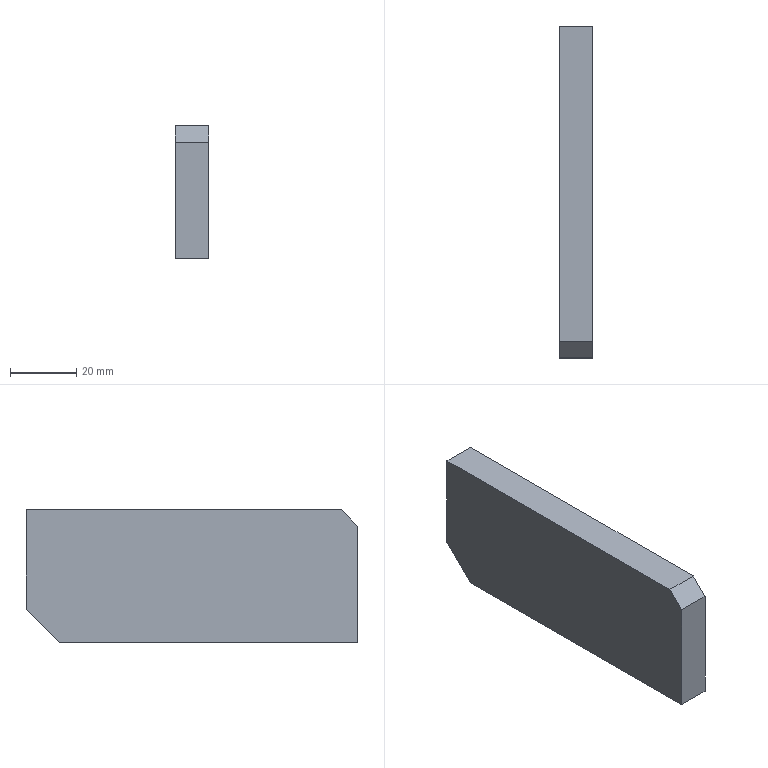Part | NX | features solid 2 | 1 solid | 8 faces | box 10 x 100 x 40 mm | volume 39375 mm3 | plane 8
STEP:
#1=CARTESIAN_POINT('',(610.,140.,-605.));
#2=VERTEX_POINT('',#1);
#3=CARTESIAN_POINT('',(610.,150.,-595.));
#4=VERTEX_POINT('',#3);
#5=CARTESIAN_POINT('',(610.,127.852,-617.148));
#6=DIRECTION('',(0.,0.7071,0.7071));
#7=VECTOR('',#6,1000.);
#8=LINE('',#5,#7);
#9=EDGE_CURVE('',#2,#4,#8,.T.);
#10=ORIENTED_EDGE('',*,*,#9,.F.);
#11=CARTESIAN_POINT('',(600.,140.,-605.));
#12=VERTEX_POINT('',#11);
#13=CARTESIAN_POINT('',(610.,140.,-605.));
#14=DIRECTION('',(1.,0.,0.));
#15=VECTOR('',#14,1000.);
#16=LINE('',#13,#15);
#17=EDGE_CURVE('',#12,#2,#16,.T.);
#18=ORIENTED_EDGE('',*,*,#17,.F.);
#19=CARTESIAN_POINT('',(600.,150.,-595.));
#20=VERTEX_POINT('',#19);
#21=CARTESIAN_POINT('',(600.,150.,-595.));
#22=DIRECTION('',(0.,-0.7071,-0.7071));
#23=VECTOR('',#22,1000.);
#24=LINE('',#21,#23);
#25=EDGE_CURVE('',#20,#12,#24,.T.);
#26=ORIENTED_EDGE('',*,*,#25,.F.);
#27=CARTESIAN_POINT('',(610.,150.,-595.));
#28=DIRECTION('',(-1.,0.,0.));
#29=VECTOR('',#28,1000.);
#30=LINE('',#27,#29);
#31=EDGE_CURVE('',#4,#20,#30,.T.);
#32=ORIENTED_EDGE('',*,*,#31,.F.);
#33=EDGE_LOOP('',(#10,#18,#26,#32));
#34=FACE_BOUND('',#33,.T.);
#35=CARTESIAN_POINT('',(610.,150.,-595.));
#36=DIRECTION('',(0.,-0.7071,0.7071));
#37=DIRECTION('',(-1.,0.,0.));
#38=AXIS2_PLACEMENT_3D('',#35,#36,#37);
#39=PLANE('',#38);
#40=ADVANCED_FACE('',(#34),#39,.F.);
#41=CARTESIAN_POINT('',(610.,55.,-565.));
#42=VERTEX_POINT('',#41);
#43=CARTESIAN_POINT('',(610.,50.,-570.));
#44=VERTEX_POINT('',#43);
#45=CARTESIAN_POINT('',(610.,65.352,-554.648));
#46=DIRECTION('',(0.,-0.7071,-0.7071));
#47=VECTOR('',#46,1000.);
#48=LINE('',#45,#47);
#49=EDGE_CURVE('',#42,#44,#48,.T.);
#50=ORIENTED_EDGE('',*,*,#49,.F.);
#51=CARTESIAN_POINT('',(600.,55.,-565.));
#52=VERTEX_POINT('',#51);
#53=CARTESIAN_POINT('',(610.,55.,-565.));
#54=DIRECTION('',(1.,0.,0.));
#55=VECTOR('',#54,1000.);
#56=LINE('',#53,#55);
#57=EDGE_CURVE('',#52,#42,#56,.T.);
#58=ORIENTED_EDGE('',*,*,#57,.F.);
#59=CARTESIAN_POINT('',(600.,50.,-570.));
#60=VERTEX_POINT('',#59);
#61=CARTESIAN_POINT('',(600.,50.,-570.));
#62=DIRECTION('',(0.,0.7071,0.7071));
#63=VECTOR('',#62,1000.);
#64=LINE('',#61,#63);
#65=EDGE_CURVE('',#60,#52,#64,.T.);
#66=ORIENTED_EDGE('',*,*,#65,.F.);
#67=CARTESIAN_POINT('',(610.,50.,-570.));
#68=DIRECTION('',(-1.,0.,0.));
#69=VECTOR('',#68,1000.);
#70=LINE('',#67,#69);
#71=EDGE_CURVE('',#44,#60,#70,.T.);
#72=ORIENTED_EDGE('',*,*,#71,.F.);
#73=EDGE_LOOP('',(#50,#58,#66,#72));
#74=FACE_BOUND('',#73,.T.);
#75=CARTESIAN_POINT('',(610.,50.,-570.));
#76=DIRECTION('',(0.,0.7071,-0.7071));
#77=DIRECTION('',(-1.,0.,0.));
#78=AXIS2_PLACEMENT_3D('',#75,#76,#77);
#79=PLANE('',#78);
#80=ADVANCED_FACE('',(#74),#79,.F.);
#81=CARTESIAN_POINT('',(600.,150.,-565.));
#82=VERTEX_POINT('',#81);
#83=CARTESIAN_POINT('',(600.,150.,-605.));
#84=DIRECTION('',(0.,0.,1.));
#85=VECTOR('',#84,1000.);
#86=LINE('',#83,#85);
#87=EDGE_CURVE('',#20,#82,#86,.T.);
#88=ORIENTED_EDGE('',*,*,#87,.F.);
#89=ORIENTED_EDGE('',*,*,#25,.T.);
#90=CARTESIAN_POINT('',(600.,50.,-605.));
#91=VERTEX_POINT('',#90);
#92=CARTESIAN_POINT('',(600.,50.,-605.));
#93=DIRECTION('',(0.,1.,0.));
#94=VECTOR('',#93,1000.);
#95=LINE('',#92,#94);
#96=EDGE_CURVE('',#91,#12,#95,.T.);
#97=ORIENTED_EDGE('',*,*,#96,.F.);
#98=CARTESIAN_POINT('',(600.,50.,-565.));
#99=DIRECTION('',(0.,0.,-1.));
#100=VECTOR('',#99,1000.);
#101=LINE('',#98,#100);
#102=EDGE_CURVE('',#60,#91,#101,.T.);
#103=ORIENTED_EDGE('',*,*,#102,.F.);
#104=ORIENTED_EDGE('',*,*,#65,.T.);
#105=CARTESIAN_POINT('',(600.,150.,-565.));
#106=DIRECTION('',(0.,-1.,0.));
#107=VECTOR('',#106,1000.);
#108=LINE('',#105,#107);
#109=EDGE_CURVE('',#82,#52,#108,.T.);
#110=ORIENTED_EDGE('',*,*,#109,.F.);
#111=EDGE_LOOP('',(#88,#89,#97,#103,#104,#110));
#112=FACE_BOUND('',#111,.T.);
#113=CARTESIAN_POINT('',(600.,111.252,-600.548));
#114=DIRECTION('',(1.,0.,0.));
#115=DIRECTION('',(0.,-1.,0.));
#116=AXIS2_PLACEMENT_3D('',#113,#114,#115);
#117=PLANE('',#116);
#118=ADVANCED_FACE('',(#112),#117,.F.);
#119=CARTESIAN_POINT('',(610.,50.,-605.));
#120=VERTEX_POINT('',#119);
#121=CARTESIAN_POINT('',(610.,50.,-605.));
#122=DIRECTION('',(0.,1.,0.));
#123=VECTOR('',#122,1000.);
#124=LINE('',#121,#123);
#125=EDGE_CURVE('',#120,#2,#124,.T.);
#126=ORIENTED_EDGE('',*,*,#125,.T.);
#127=ORIENTED_EDGE('',*,*,#9,.T.);
#128=CARTESIAN_POINT('',(610.,150.,-565.));
#129=VERTEX_POINT('',#128);
#130=CARTESIAN_POINT('',(610.,150.,-605.));
#131=DIRECTION('',(0.,0.,1.));
#132=VECTOR('',#131,1000.);
#133=LINE('',#130,#132);
#134=EDGE_CURVE('',#4,#129,#133,.T.);
#135=ORIENTED_EDGE('',*,*,#134,.T.);
#136=CARTESIAN_POINT('',(610.,150.,-565.));
#137=DIRECTION('',(0.,-1.,0.));
#138=VECTOR('',#137,1000.);
#139=LINE('',#136,#138);
#140=EDGE_CURVE('',#129,#42,#139,.T.);
#141=ORIENTED_EDGE('',*,*,#140,.T.);
#142=ORIENTED_EDGE('',*,*,#49,.T.);
#143=CARTESIAN_POINT('',(610.,50.,-565.));
#144=DIRECTION('',(0.,0.,-1.));
#145=VECTOR('',#144,1000.);
#146=LINE('',#143,#145);
#147=EDGE_CURVE('',#44,#120,#146,.T.);
#148=ORIENTED_EDGE('',*,*,#147,.T.);
#149=EDGE_LOOP('',(#126,#127,#135,#141,#142,#148));
#150=FACE_BOUND('',#149,.T.);
#151=CARTESIAN_POINT('',(610.,111.252,-600.548));
#152=DIRECTION('',(1.,0.,0.));
#153=DIRECTION('',(0.,-1.,0.));
#154=AXIS2_PLACEMENT_3D('',#151,#152,#153);
#155=PLANE('',#154);
#156=ADVANCED_FACE('',(#150),#155,.T.);
#157=ORIENTED_EDGE('',*,*,#109,.T.);
#158=ORIENTED_EDGE('',*,*,#57,.T.);
#159=ORIENTED_EDGE('',*,*,#140,.F.);
#160=CARTESIAN_POINT('',(610.,150.,-565.));
#161=DIRECTION('',(-1.,0.,0.));
#162=VECTOR('',#161,1000.);
#163=LINE('',#160,#162);
#164=EDGE_CURVE('',#129,#82,#163,.T.);
#165=ORIENTED_EDGE('',*,*,#164,.T.);
#166=EDGE_LOOP('',(#157,#158,#159,#165));
#167=FACE_BOUND('',#166,.T.);
#168=CARTESIAN_POINT('',(610.,150.,-565.));
#169=DIRECTION('',(0.,0.,-1.));
#170=DIRECTION('',(-1.,0.,0.));
#171=AXIS2_PLACEMENT_3D('',#168,#169,#170);
#172=PLANE('',#171);
#173=ADVANCED_FACE('',(#167),#172,.F.);
#174=ORIENTED_EDGE('',*,*,#134,.F.);
#175=ORIENTED_EDGE('',*,*,#31,.T.);
#176=ORIENTED_EDGE('',*,*,#87,.T.);
#177=ORIENTED_EDGE('',*,*,#164,.F.);
#178=EDGE_LOOP('',(#174,#175,#176,#177));
#179=FACE_BOUND('',#178,.T.);
#180=CARTESIAN_POINT('',(610.,150.,-605.));
#181=DIRECTION('',(0.,-1.,0.));
#182=DIRECTION('',(-1.,0.,0.));
#183=AXIS2_PLACEMENT_3D('',#180,#181,#182);
#184=PLANE('',#183);
#185=ADVANCED_FACE('',(#179),#184,.F.);
#186=ORIENTED_EDGE('',*,*,#96,.T.);
#187=ORIENTED_EDGE('',*,*,#17,.T.);
#188=ORIENTED_EDGE('',*,*,#125,.F.);
#189=CARTESIAN_POINT('',(610.,50.,-605.));
#190=DIRECTION('',(-1.,0.,0.));
#191=VECTOR('',#190,1000.);
#192=LINE('',#189,#191);
#193=EDGE_CURVE('',#120,#91,#192,.T.);
#194=ORIENTED_EDGE('',*,*,#193,.T.);
#195=EDGE_LOOP('',(#186,#187,#188,#194));
#196=FACE_BOUND('',#195,.T.);
#197=CARTESIAN_POINT('',(610.,50.,-605.));
#198=DIRECTION('',(0.,0.,1.));
#199=DIRECTION('',(0.,-1.,0.));
#200=AXIS2_PLACEMENT_3D('',#197,#198,#199);
#201=PLANE('',#200);
#202=ADVANCED_FACE('',(#196),#201,.F.);
#203=ORIENTED_EDGE('',*,*,#147,.F.);
#204=ORIENTED_EDGE('',*,*,#71,.T.);
#205=ORIENTED_EDGE('',*,*,#102,.T.);
#206=ORIENTED_EDGE('',*,*,#193,.F.);
#207=EDGE_LOOP('',(#203,#204,#205,#206));
#208=FACE_BOUND('',#207,.T.);
#209=CARTESIAN_POINT('',(610.,50.,-565.));
#210=DIRECTION('',(0.,1.,0.));
#211=DIRECTION('',(0.,0.,-1.));
#212=AXIS2_PLACEMENT_3D('',#209,#210,#211);
#213=PLANE('',#212);
#214=ADVANCED_FACE('',(#208),#213,.F.);
#215=CLOSED_SHELL('',(#40,#80,#118,#156,#173,#185,#202,#214));
#216=MANIFOLD_SOLID_BREP('',#215);
#217=(LENGTH_UNIT()NAMED_UNIT(*)SI_UNIT(.MILLI.,.METRE.));
#218=UNCERTAINTY_MEASURE_WITH_UNIT(LENGTH_MEASURE(0.00001),#217,'','');
#219=(NAMED_UNIT(*)PLANE_ANGLE_UNIT()SI_UNIT($,.RADIAN.));
#220=(NAMED_UNIT(*)SI_UNIT($,.STERADIAN.)SOLID_ANGLE_UNIT());
#221=(GEOMETRIC_REPRESENTATION_CONTEXT(3)GLOBAL_UNCERTAINTY_ASSIGNED_CONTEXT((#218))GLOBAL_UNIT_ASSIGNED_CONTEXT((#217,#219,#220))REPRESENTATION_CONTEXT('',''));
#222=ADVANCED_BREP_SHAPE_REPRESENTATION('',(#216),#221);